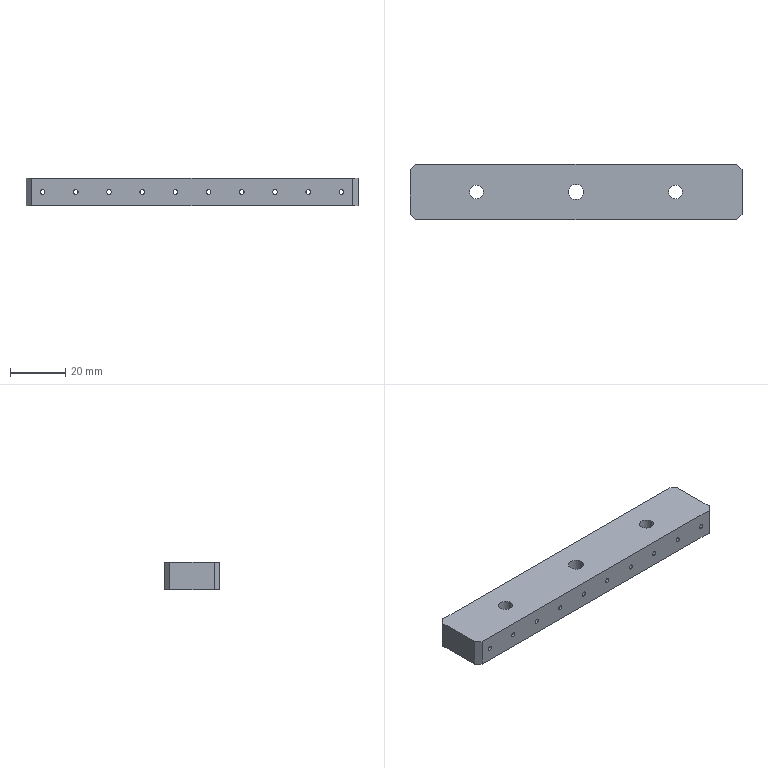Part | SolidWorks | features HoleWzd 2, ICE 2, Chamfer 1, Extrusion 1, LPattern 1 | 1 solid | 66 faces | box 120 x 20 x 10 mm | volume 22814 mm3 | cylinder 46 | plane 20 | commonest cylinder face diameters 1.65 x20 2.18 x20 5 x4 5.5 x2